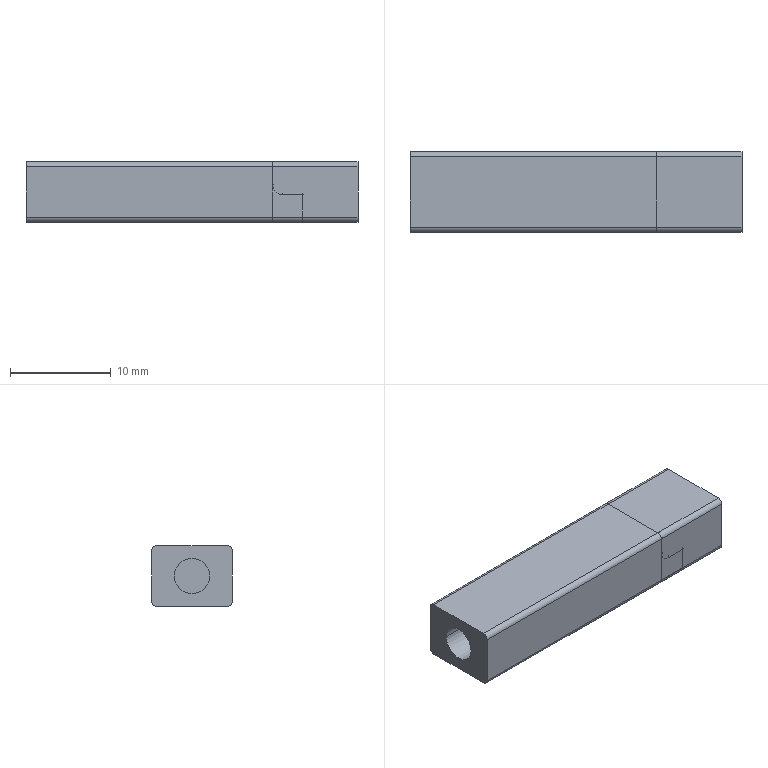Part | 2 solids | 73 faces | box 33 x 8 x 6 mm | volume 1614 mm3 | cylinder 32 | plane 19 | torus 10 | sphere 8 | spline 4 | commonest cylinder face diameters 1 x27 2 x3 3.5 x2